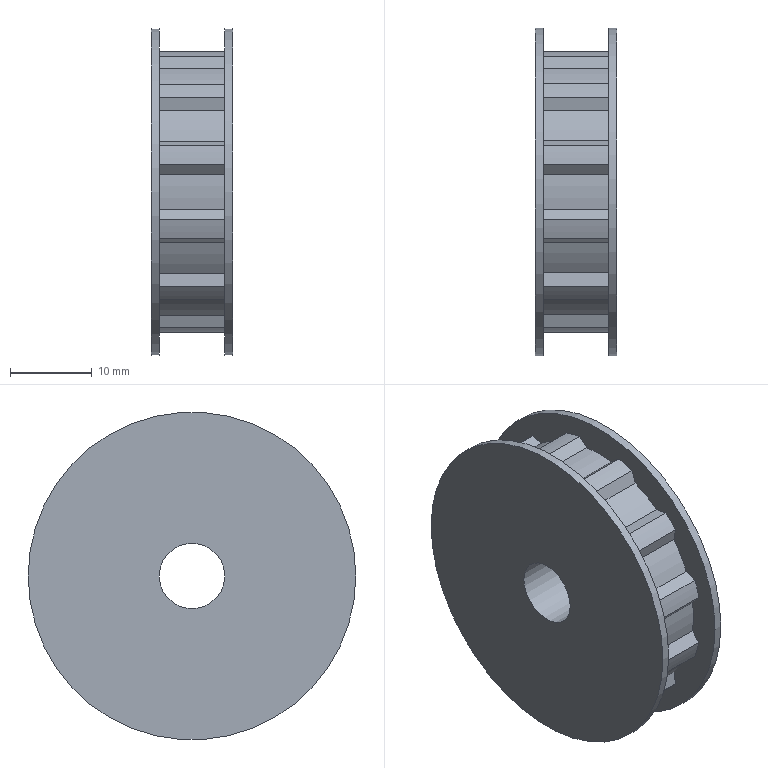Part | NX | features DATUM_CSYS 3, EXTRUDE 2, SKETCH 2, Container 1, EXTRACT_BODY 1, Geometry Instance 1, UNITE 1 | 1 solid | 55 faces | box 10 x 40 x 40 mm | volume 9050 mm3 | plane 28 | cylinder 27 | commonest cylinder face diameters 32.525 x12 35 x12 40 x2 8 x1